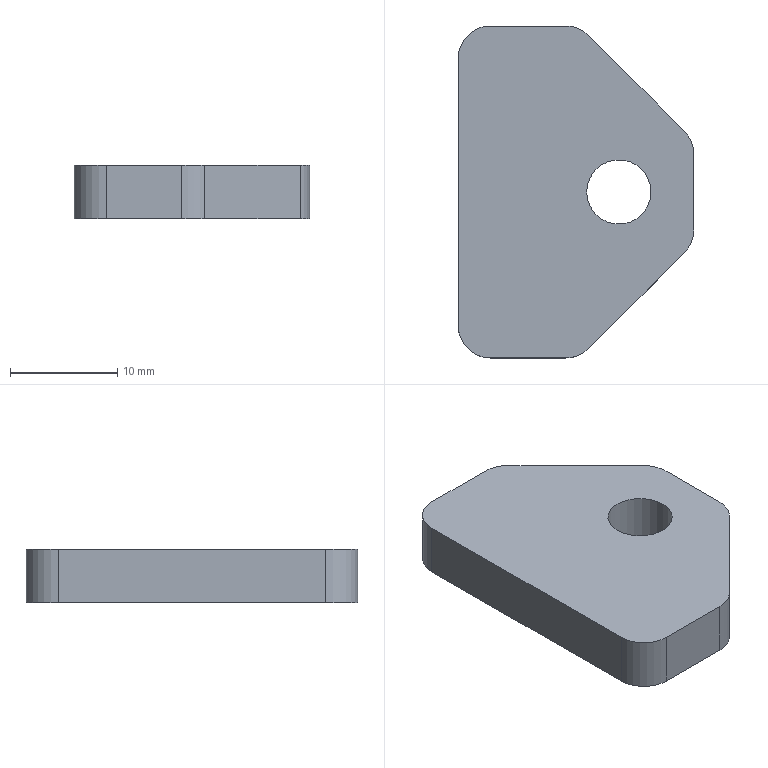Part | NX | features DIE-23 2 | 1 solid | 15 faces | box 22 x 31 x 5 mm | volume 2672 mm3 | plane 8 | cylinder 7 | commonest cylinder face diameters 6 x6 6.007 x1
STEP:
#1=CARTESIAN_POINT('',(2452.36,-823.273,843.716));
#2=VERTEX_POINT('',#1);
#3=CARTESIAN_POINT('',(2445.31,-823.273,843.716));
#4=VERTEX_POINT('',#3);
#5=CARTESIAN_POINT('',(2447.81,-823.273,843.716));
#6=DIRECTION('',(-1.,0.,0.));
#7=VECTOR('',#6,1000.);
#8=LINE('',#5,#7);
#9=EDGE_CURVE('',#2,#4,#8,.T.);
#10=ORIENTED_EDGE('',*,*,#9,.F.);
#11=CARTESIAN_POINT('',(2452.36,-823.273,838.716));
#12=VERTEX_POINT('',#11);
#13=CARTESIAN_POINT('',(2452.36,-823.273,838.716));
#14=DIRECTION('',(0.,0.,1.));
#15=VECTOR('',#14,1000.);
#16=LINE('',#13,#15);
#17=EDGE_CURVE('',#12,#2,#16,.T.);
#18=ORIENTED_EDGE('',*,*,#17,.F.);
#19=CARTESIAN_POINT('',(2445.31,-823.273,838.716));
#20=VERTEX_POINT('',#19);
#21=CARTESIAN_POINT('',(2447.81,-823.273,838.716));
#22=DIRECTION('',(-1.,0.,0.));
#23=VECTOR('',#22,1000.);
#24=LINE('',#21,#23);
#25=EDGE_CURVE('',#12,#20,#24,.T.);
#26=ORIENTED_EDGE('',*,*,#25,.T.);
#27=CARTESIAN_POINT('',(2445.31,-823.273,838.716));
#28=DIRECTION('',(0.,0.,1.));
#29=VECTOR('',#28,1000.);
#30=LINE('',#27,#29);
#31=EDGE_CURVE('',#20,#4,#30,.T.);
#32=ORIENTED_EDGE('',*,*,#31,.T.);
#33=EDGE_LOOP('',(#10,#18,#26,#32));
#34=FACE_BOUND('',#33,.T.);
#35=CARTESIAN_POINT('',(2447.81,-823.273,838.716));
#36=DIRECTION('',(0.,1.,0.));
#37=DIRECTION('',(0.,0.,1.));
#38=AXIS2_PLACEMENT_3D('',#35,#36,#37);
#39=PLANE('',#38);
#40=ADVANCED_FACE('',(#34),#39,.T.);
#41=CARTESIAN_POINT('',(2454.481,-824.152,843.716));
#42=VERTEX_POINT('',#41);
#43=CARTESIAN_POINT('',(2452.36,-826.273,843.716));
#44=DIRECTION('',(0.,0.,-1.));
#45=DIRECTION('',(-1.,0.,0.));
#46=AXIS2_PLACEMENT_3D('',#43,#44,#45);
#47=CIRCLE('',#46,3.);
#48=EDGE_CURVE('',#2,#42,#47,.T.);
#49=ORIENTED_EDGE('',*,*,#48,.T.);
#50=CARTESIAN_POINT('',(2454.481,-824.152,838.716));
#51=VERTEX_POINT('',#50);
#52=CARTESIAN_POINT('',(2454.481,-824.152,838.716));
#53=DIRECTION('',(0.,0.,1.));
#54=VECTOR('',#53,1000.);
#55=LINE('',#52,#54);
#56=EDGE_CURVE('',#51,#42,#55,.T.);
#57=ORIENTED_EDGE('',*,*,#56,.F.);
#58=CARTESIAN_POINT('',(2452.36,-826.273,838.716));
#59=DIRECTION('',(0.,0.,-1.));
#60=DIRECTION('',(-1.,0.,0.));
#61=AXIS2_PLACEMENT_3D('',#58,#59,#60);
#62=CIRCLE('',#61,3.);
#63=EDGE_CURVE('',#12,#51,#62,.T.);
#64=ORIENTED_EDGE('',*,*,#63,.F.);
#65=ORIENTED_EDGE('',*,*,#17,.T.);
#66=EDGE_LOOP('',(#49,#57,#64,#65));
#67=FACE_BOUND('',#66,.T.);
#68=CARTESIAN_POINT('',(2452.36,-826.273,838.716));
#69=DIRECTION('',(0.,0.,1.));
#70=DIRECTION('',(1.,0.,0.));
#71=AXIS2_PLACEMENT_3D('',#68,#69,#70);
#72=CYLINDRICAL_SURFACE('',#71,3.);
#73=ADVANCED_FACE('',(#67),#72,.T.);
#74=CARTESIAN_POINT('',(2463.431,-833.102,843.716));
#75=VERTEX_POINT('',#74);
#76=CARTESIAN_POINT('',(2458.456,-828.127,843.716));
#77=DIRECTION('',(0.7071,-0.7071,0.));
#78=VECTOR('',#77,1000.);
#79=LINE('',#76,#78);
#80=EDGE_CURVE('',#42,#75,#79,.T.);
#81=ORIENTED_EDGE('',*,*,#80,.T.);
#82=CARTESIAN_POINT('',(2463.431,-833.102,838.716));
#83=VERTEX_POINT('',#82);
#84=CARTESIAN_POINT('',(2463.431,-833.102,838.716));
#85=DIRECTION('',(0.,0.,1.));
#86=VECTOR('',#85,1000.);
#87=LINE('',#84,#86);
#88=EDGE_CURVE('',#83,#75,#87,.T.);
#89=ORIENTED_EDGE('',*,*,#88,.F.);
#90=CARTESIAN_POINT('',(2458.456,-828.127,838.716));
#91=DIRECTION('',(0.7071,-0.7071,0.));
#92=VECTOR('',#91,1000.);
#93=LINE('',#90,#92);
#94=EDGE_CURVE('',#51,#83,#93,.T.);
#95=ORIENTED_EDGE('',*,*,#94,.F.);
#96=ORIENTED_EDGE('',*,*,#56,.T.);
#97=EDGE_LOOP('',(#81,#89,#95,#96));
#98=FACE_BOUND('',#97,.T.);
#99=CARTESIAN_POINT('',(2458.456,-828.127,838.716));
#100=DIRECTION('',(-0.7071,-0.7071,0.));
#101=DIRECTION('',(0.7071,-0.7071,0.));
#102=AXIS2_PLACEMENT_3D('',#99,#100,#101);
#103=PLANE('',#102);
#104=ADVANCED_FACE('',(#98),#103,.F.);
#105=CARTESIAN_POINT('',(2464.31,-835.223,843.716));
#106=VERTEX_POINT('',#105);
#107=CARTESIAN_POINT('',(2461.31,-835.223,843.716));
#108=DIRECTION('',(0.,0.,-1.));
#109=DIRECTION('',(-1.,0.,0.));
#110=AXIS2_PLACEMENT_3D('',#107,#108,#109);
#111=CIRCLE('',#110,3.);
#112=EDGE_CURVE('',#75,#106,#111,.T.);
#113=ORIENTED_EDGE('',*,*,#112,.T.);
#114=CARTESIAN_POINT('',(2464.31,-835.223,838.716));
#115=VERTEX_POINT('',#114);
#116=CARTESIAN_POINT('',(2464.31,-835.223,838.716));
#117=DIRECTION('',(0.,0.,1.));
#118=VECTOR('',#117,1000.);
#119=LINE('',#116,#118);
#120=EDGE_CURVE('',#115,#106,#119,.T.);
#121=ORIENTED_EDGE('',*,*,#120,.F.);
#122=CARTESIAN_POINT('',(2461.31,-835.223,838.716));
#123=DIRECTION('',(0.,0.,-1.));
#124=DIRECTION('',(-1.,0.,0.));
#125=AXIS2_PLACEMENT_3D('',#122,#123,#124);
#126=CIRCLE('',#125,3.);
#127=EDGE_CURVE('',#83,#115,#126,.T.);
#128=ORIENTED_EDGE('',*,*,#127,.F.);
#129=ORIENTED_EDGE('',*,*,#88,.T.);
#130=EDGE_LOOP('',(#113,#121,#128,#129));
#131=FACE_BOUND('',#130,.T.);
#132=CARTESIAN_POINT('',(2461.31,-835.223,838.716));
#133=DIRECTION('',(0.,0.,1.));
#134=DIRECTION('',(1.,0.,0.));
#135=AXIS2_PLACEMENT_3D('',#132,#133,#134);
#136=CYLINDRICAL_SURFACE('',#135,3.);
#137=ADVANCED_FACE('',(#131),#136,.T.);
#138=CARTESIAN_POINT('',(2464.31,-842.324,843.716));
#139=VERTEX_POINT('',#138);
#140=CARTESIAN_POINT('',(2464.31,-838.773,843.716));
#141=DIRECTION('',(0.,1.,0.));
#142=VECTOR('',#141,1000.);
#143=LINE('',#140,#142);
#144=EDGE_CURVE('',#139,#106,#143,.T.);
#145=ORIENTED_EDGE('',*,*,#144,.F.);
#146=CARTESIAN_POINT('',(2464.31,-842.324,838.716));
#147=VERTEX_POINT('',#146);
#148=CARTESIAN_POINT('',(2464.31,-842.324,838.716));
#149=DIRECTION('',(0.,0.,1.));
#150=VECTOR('',#149,1000.);
#151=LINE('',#148,#150);
#152=EDGE_CURVE('',#147,#139,#151,.T.);
#153=ORIENTED_EDGE('',*,*,#152,.F.);
#154=CARTESIAN_POINT('',(2464.31,-838.773,838.716));
#155=DIRECTION('',(0.,1.,0.));
#156=VECTOR('',#155,1000.);
#157=LINE('',#154,#156);
#158=EDGE_CURVE('',#147,#115,#157,.T.);
#159=ORIENTED_EDGE('',*,*,#158,.T.);
#160=ORIENTED_EDGE('',*,*,#120,.T.);
#161=EDGE_LOOP('',(#145,#153,#159,#160));
#162=FACE_BOUND('',#161,.T.);
#163=CARTESIAN_POINT('',(2464.31,-838.773,838.716));
#164=DIRECTION('',(1.,0.,0.));
#165=DIRECTION('',(0.,0.,-1.));
#166=AXIS2_PLACEMENT_3D('',#163,#164,#165);
#167=PLANE('',#166);
#168=ADVANCED_FACE('',(#162),#167,.T.);
#169=CARTESIAN_POINT('',(2463.431,-844.445,843.716));
#170=VERTEX_POINT('',#169);
#171=CARTESIAN_POINT('',(2461.31,-842.324,843.716));
#172=DIRECTION('',(0.,0.,-1.));
#173=DIRECTION('',(-1.,0.,0.));
#174=AXIS2_PLACEMENT_3D('',#171,#172,#173);
#175=CIRCLE('',#174,3.);
#176=EDGE_CURVE('',#139,#170,#175,.T.);
#177=ORIENTED_EDGE('',*,*,#176,.T.);
#178=CARTESIAN_POINT('',(2463.431,-844.445,838.716));
#179=VERTEX_POINT('',#178);
#180=CARTESIAN_POINT('',(2463.431,-844.445,838.716));
#181=DIRECTION('',(0.,0.,1.));
#182=VECTOR('',#181,1000.);
#183=LINE('',#180,#182);
#184=EDGE_CURVE('',#179,#170,#183,.T.);
#185=ORIENTED_EDGE('',*,*,#184,.F.);
#186=CARTESIAN_POINT('',(2461.31,-842.324,838.716));
#187=DIRECTION('',(0.,0.,-1.));
#188=DIRECTION('',(-1.,0.,0.));
#189=AXIS2_PLACEMENT_3D('',#186,#187,#188);
#190=CIRCLE('',#189,3.);
#191=EDGE_CURVE('',#147,#179,#190,.T.);
#192=ORIENTED_EDGE('',*,*,#191,.F.);
#193=ORIENTED_EDGE('',*,*,#152,.T.);
#194=EDGE_LOOP('',(#177,#185,#192,#193));
#195=FACE_BOUND('',#194,.T.);
#196=CARTESIAN_POINT('',(2461.31,-842.324,838.716));
#197=DIRECTION('',(0.,0.,1.));
#198=DIRECTION('',(1.,0.,0.));
#199=AXIS2_PLACEMENT_3D('',#196,#197,#198);
#200=CYLINDRICAL_SURFACE('',#199,3.);
#201=ADVANCED_FACE('',(#195),#200,.T.);
#202=CARTESIAN_POINT('',(2454.481,-853.395,843.716));
#203=VERTEX_POINT('',#202);
#204=CARTESIAN_POINT('',(2458.456,-849.42,843.716));
#205=DIRECTION('',(-0.7071,-0.7071,0.));
#206=VECTOR('',#205,1000.);
#207=LINE('',#204,#206);
#208=EDGE_CURVE('',#170,#203,#207,.T.);
#209=ORIENTED_EDGE('',*,*,#208,.T.);
#210=CARTESIAN_POINT('',(2454.481,-853.395,838.716));
#211=VERTEX_POINT('',#210);
#212=CARTESIAN_POINT('',(2454.481,-853.395,838.716));
#213=DIRECTION('',(0.,0.,1.));
#214=VECTOR('',#213,1000.);
#215=LINE('',#212,#214);
#216=EDGE_CURVE('',#211,#203,#215,.T.);
#217=ORIENTED_EDGE('',*,*,#216,.F.);
#218=CARTESIAN_POINT('',(2458.456,-849.42,838.716));
#219=DIRECTION('',(-0.7071,-0.7071,0.));
#220=VECTOR('',#219,1000.);
#221=LINE('',#218,#220);
#222=EDGE_CURVE('',#179,#211,#221,.T.);
#223=ORIENTED_EDGE('',*,*,#222,.F.);
#224=ORIENTED_EDGE('',*,*,#184,.T.);
#225=EDGE_LOOP('',(#209,#217,#223,#224));
#226=FACE_BOUND('',#225,.T.);
#227=CARTESIAN_POINT('',(2458.456,-849.42,838.716));
#228=DIRECTION('',(-0.7071,0.7071,0.));
#229=DIRECTION('',(-0.7071,-0.7071,0.));
#230=AXIS2_PLACEMENT_3D('',#227,#228,#229);
#231=PLANE('',#230);
#232=ADVANCED_FACE('',(#226),#231,.F.);
#233=CARTESIAN_POINT('',(2452.36,-854.273,843.716));
#234=VERTEX_POINT('',#233);
#235=CARTESIAN_POINT('',(2452.36,-851.273,843.716));
#236=DIRECTION('',(0.,0.,-1.));
#237=DIRECTION('',(-1.,0.,0.));
#238=AXIS2_PLACEMENT_3D('',#235,#236,#237);
#239=CIRCLE('',#238,3.);
#240=EDGE_CURVE('',#203,#234,#239,.T.);
#241=ORIENTED_EDGE('',*,*,#240,.T.);
#242=CARTESIAN_POINT('',(2452.36,-854.273,838.716));
#243=VERTEX_POINT('',#242);
#244=CARTESIAN_POINT('',(2452.36,-854.273,838.716));
#245=DIRECTION('',(0.,0.,1.));
#246=VECTOR('',#245,1000.);
#247=LINE('',#244,#246);
#248=EDGE_CURVE('',#243,#234,#247,.T.);
#249=ORIENTED_EDGE('',*,*,#248,.F.);
#250=CARTESIAN_POINT('',(2452.36,-851.273,838.716));
#251=DIRECTION('',(0.,0.,-1.));
#252=DIRECTION('',(-1.,0.,0.));
#253=AXIS2_PLACEMENT_3D('',#250,#251,#252);
#254=CIRCLE('',#253,3.);
#255=EDGE_CURVE('',#211,#243,#254,.T.);
#256=ORIENTED_EDGE('',*,*,#255,.F.);
#257=ORIENTED_EDGE('',*,*,#216,.T.);
#258=EDGE_LOOP('',(#241,#249,#256,#257));
#259=FACE_BOUND('',#258,.T.);
#260=CARTESIAN_POINT('',(2452.36,-851.273,838.716));
#261=DIRECTION('',(0.,0.,1.));
#262=DIRECTION('',(1.,0.,0.));
#263=AXIS2_PLACEMENT_3D('',#260,#261,#262);
#264=CYLINDRICAL_SURFACE('',#263,3.);
#265=ADVANCED_FACE('',(#259),#264,.T.);
#266=CARTESIAN_POINT('',(2445.31,-854.273,843.716));
#267=VERTEX_POINT('',#266);
#268=CARTESIAN_POINT('',(2447.81,-854.273,843.716));
#269=DIRECTION('',(1.,0.,0.));
#270=VECTOR('',#269,1000.);
#271=LINE('',#268,#270);
#272=EDGE_CURVE('',#267,#234,#271,.T.);
#273=ORIENTED_EDGE('',*,*,#272,.F.);
#274=CARTESIAN_POINT('',(2445.31,-854.273,838.716));
#275=VERTEX_POINT('',#274);
#276=CARTESIAN_POINT('',(2445.31,-854.273,838.716));
#277=DIRECTION('',(0.,0.,1.));
#278=VECTOR('',#277,1000.);
#279=LINE('',#276,#278);
#280=EDGE_CURVE('',#275,#267,#279,.T.);
#281=ORIENTED_EDGE('',*,*,#280,.F.);
#282=CARTESIAN_POINT('',(2447.81,-854.273,838.716));
#283=DIRECTION('',(1.,0.,0.));
#284=VECTOR('',#283,1000.);
#285=LINE('',#282,#284);
#286=EDGE_CURVE('',#275,#243,#285,.T.);
#287=ORIENTED_EDGE('',*,*,#286,.T.);
#288=ORIENTED_EDGE('',*,*,#248,.T.);
#289=EDGE_LOOP('',(#273,#281,#287,#288));
#290=FACE_BOUND('',#289,.T.);
#291=CARTESIAN_POINT('',(2447.81,-854.273,838.716));
#292=DIRECTION('',(0.,-1.,0.));
#293=DIRECTION('',(0.,0.,-1.));
#294=AXIS2_PLACEMENT_3D('',#291,#292,#293);
#295=PLANE('',#294);
#296=ADVANCED_FACE('',(#290),#295,.T.);
#297=CARTESIAN_POINT('',(2442.31,-851.273,843.716));
#298=VERTEX_POINT('',#297);
#299=CARTESIAN_POINT('',(2445.31,-851.273,843.716));
#300=DIRECTION('',(0.,0.,-1.));
#301=DIRECTION('',(-1.,0.,0.));
#302=AXIS2_PLACEMENT_3D('',#299,#300,#301);
#303=CIRCLE('',#302,3.);
#304=EDGE_CURVE('',#267,#298,#303,.T.);
#305=ORIENTED_EDGE('',*,*,#304,.T.);
#306=CARTESIAN_POINT('',(2442.31,-851.273,838.716));
#307=VERTEX_POINT('',#306);
#308=CARTESIAN_POINT('',(2442.31,-851.273,838.716));
#309=DIRECTION('',(0.,0.,1.));
#310=VECTOR('',#309,1000.);
#311=LINE('',#308,#310);
#312=EDGE_CURVE('',#307,#298,#311,.T.);
#313=ORIENTED_EDGE('',*,*,#312,.F.);
#314=CARTESIAN_POINT('',(2445.31,-851.273,838.716));
#315=DIRECTION('',(0.,0.,-1.));
#316=DIRECTION('',(-1.,0.,0.));
#317=AXIS2_PLACEMENT_3D('',#314,#315,#316);
#318=CIRCLE('',#317,3.);
#319=EDGE_CURVE('',#275,#307,#318,.T.);
#320=ORIENTED_EDGE('',*,*,#319,.F.);
#321=ORIENTED_EDGE('',*,*,#280,.T.);
#322=EDGE_LOOP('',(#305,#313,#320,#321));
#323=FACE_BOUND('',#322,.T.);
#324=CARTESIAN_POINT('',(2445.31,-851.273,838.716));
#325=DIRECTION('',(0.,0.,1.));
#326=DIRECTION('',(1.,0.,0.));
#327=AXIS2_PLACEMENT_3D('',#324,#325,#326);
#328=CYLINDRICAL_SURFACE('',#327,3.);
#329=ADVANCED_FACE('',(#323),#328,.T.);
#330=CARTESIAN_POINT('',(2442.31,-826.273,843.716));
#331=VERTEX_POINT('',#330);
#332=CARTESIAN_POINT('',(2442.31,-838.773,843.716));
#333=DIRECTION('',(0.,-1.,0.));
#334=VECTOR('',#333,1000.);
#335=LINE('',#332,#334);
#336=EDGE_CURVE('',#331,#298,#335,.T.);
#337=ORIENTED_EDGE('',*,*,#336,.F.);
#338=CARTESIAN_POINT('',(2442.31,-826.273,838.716));
#339=VERTEX_POINT('',#338);
#340=CARTESIAN_POINT('',(2442.31,-826.273,838.716));
#341=DIRECTION('',(0.,0.,1.));
#342=VECTOR('',#341,1000.);
#343=LINE('',#340,#342);
#344=EDGE_CURVE('',#339,#331,#343,.T.);
#345=ORIENTED_EDGE('',*,*,#344,.F.);
#346=CARTESIAN_POINT('',(2442.31,-838.773,838.716));
#347=DIRECTION('',(0.,-1.,0.));
#348=VECTOR('',#347,1000.);
#349=LINE('',#346,#348);
#350=EDGE_CURVE('',#339,#307,#349,.T.);
#351=ORIENTED_EDGE('',*,*,#350,.T.);
#352=ORIENTED_EDGE('',*,*,#312,.T.);
#353=EDGE_LOOP('',(#337,#345,#351,#352));
#354=FACE_BOUND('',#353,.T.);
#355=CARTESIAN_POINT('',(2442.31,-838.773,838.716));
#356=DIRECTION('',(-1.,0.,0.));
#357=DIRECTION('',(0.,0.,1.));
#358=AXIS2_PLACEMENT_3D('',#355,#356,#357);
#359=PLANE('',#358);
#360=ADVANCED_FACE('',(#354),#359,.T.);
#361=CARTESIAN_POINT('',(2454.306,-838.773,838.716));
#362=VERTEX_POINT('',#361);
#363=CARTESIAN_POINT('',(2457.31,-838.773,838.716));
#364=DIRECTION('',(0.,0.,-1.));
#365=DIRECTION('',(-1.,0.,0.));
#366=AXIS2_PLACEMENT_3D('',#363,#364,#365);
#367=CIRCLE('',#366,3.003);
#368=EDGE_CURVE('',#362,#362,#367,.T.);
#369=ORIENTED_EDGE('',*,*,#368,.T.);
#370=EDGE_LOOP('',(#369));
#371=FACE_BOUND('',#370,.T.);
#372=CARTESIAN_POINT('',(2454.306,-838.773,843.716));
#373=VERTEX_POINT('',#372);
#374=CARTESIAN_POINT('',(2457.31,-838.773,843.716));
#375=DIRECTION('',(0.,0.,-1.));
#376=DIRECTION('',(-1.,0.,0.));
#377=AXIS2_PLACEMENT_3D('',#374,#375,#376);
#378=CIRCLE('',#377,3.003);
#379=EDGE_CURVE('',#373,#373,#378,.T.);
#380=ORIENTED_EDGE('',*,*,#379,.F.);
#381=EDGE_LOOP('',(#380));
#382=FACE_BOUND('',#381,.T.);
#383=CARTESIAN_POINT('',(2457.31,-838.773,838.716));
#384=DIRECTION('',(0.,0.,1.));
#385=DIRECTION('',(1.,0.,0.));
#386=AXIS2_PLACEMENT_3D('',#383,#384,#385);
#387=CYLINDRICAL_SURFACE('',#386,3.003);
#388=ADVANCED_FACE('',(#371,#382),#387,.F.);
#389=CARTESIAN_POINT('',(2445.31,-826.273,843.716));
#390=DIRECTION('',(0.,0.,-1.));
#391=DIRECTION('',(-1.,0.,0.));
#392=AXIS2_PLACEMENT_3D('',#389,#390,#391);
#393=CIRCLE('',#392,3.);
#394=EDGE_CURVE('',#331,#4,#393,.T.);
#395=ORIENTED_EDGE('',*,*,#394,.T.);
#396=ORIENTED_EDGE('',*,*,#31,.F.);
#397=CARTESIAN_POINT('',(2445.31,-826.273,838.716));
#398=DIRECTION('',(0.,0.,-1.));
#399=DIRECTION('',(-1.,0.,0.));
#400=AXIS2_PLACEMENT_3D('',#397,#398,#399);
#401=CIRCLE('',#400,3.);
#402=EDGE_CURVE('',#339,#20,#401,.T.);
#403=ORIENTED_EDGE('',*,*,#402,.F.);
#404=ORIENTED_EDGE('',*,*,#344,.T.);
#405=EDGE_LOOP('',(#395,#396,#403,#404));
#406=FACE_BOUND('',#405,.T.);
#407=CARTESIAN_POINT('',(2445.31,-826.273,838.716));
#408=DIRECTION('',(0.,0.,1.));
#409=DIRECTION('',(1.,0.,0.));
#410=AXIS2_PLACEMENT_3D('',#407,#408,#409);
#411=CYLINDRICAL_SURFACE('',#410,3.);
#412=ADVANCED_FACE('',(#406),#411,.T.);
#413=ORIENTED_EDGE('',*,*,#368,.F.);
#414=EDGE_LOOP('',(#413));
#415=FACE_BOUND('',#414,.T.);
#416=ORIENTED_EDGE('',*,*,#25,.F.);
#417=ORIENTED_EDGE('',*,*,#63,.T.);
#418=ORIENTED_EDGE('',*,*,#94,.T.);
#419=ORIENTED_EDGE('',*,*,#127,.T.);
#420=ORIENTED_EDGE('',*,*,#158,.F.);
#421=ORIENTED_EDGE('',*,*,#191,.T.);
#422=ORIENTED_EDGE('',*,*,#222,.T.);
#423=ORIENTED_EDGE('',*,*,#255,.T.);
#424=ORIENTED_EDGE('',*,*,#286,.F.);
#425=ORIENTED_EDGE('',*,*,#319,.T.);
#426=ORIENTED_EDGE('',*,*,#350,.F.);
#427=ORIENTED_EDGE('',*,*,#402,.T.);
#428=EDGE_LOOP('',(#416,#417,#418,#419,#420,#421,#422,#423,#424,#425,#426,#427));
#429=FACE_BOUND('',#428,.T.);
#430=CARTESIAN_POINT('',(2447.81,-838.773,838.716));
#431=DIRECTION('',(0.,0.,-1.));
#432=DIRECTION('',(-1.,0.,0.));
#433=AXIS2_PLACEMENT_3D('',#430,#431,#432);
#434=PLANE('',#433);
#435=ADVANCED_FACE('',(#415,#429),#434,.T.);
#436=ORIENTED_EDGE('',*,*,#379,.T.);
#437=EDGE_LOOP('',(#436));
#438=FACE_BOUND('',#437,.T.);
#439=ORIENTED_EDGE('',*,*,#9,.T.);
#440=ORIENTED_EDGE('',*,*,#394,.F.);
#441=ORIENTED_EDGE('',*,*,#336,.T.);
#442=ORIENTED_EDGE('',*,*,#304,.F.);
#443=ORIENTED_EDGE('',*,*,#272,.T.);
#444=ORIENTED_EDGE('',*,*,#240,.F.);
#445=ORIENTED_EDGE('',*,*,#208,.F.);
#446=ORIENTED_EDGE('',*,*,#176,.F.);
#447=ORIENTED_EDGE('',*,*,#144,.T.);
#448=ORIENTED_EDGE('',*,*,#112,.F.);
#449=ORIENTED_EDGE('',*,*,#80,.F.);
#450=ORIENTED_EDGE('',*,*,#48,.F.);
#451=EDGE_LOOP('',(#439,#440,#441,#442,#443,#444,#445,#446,#447,#448,#449,#450));
#452=FACE_BOUND('',#451,.T.);
#453=CARTESIAN_POINT('',(2447.81,-838.773,843.716));
#454=DIRECTION('',(0.,0.,-1.));
#455=DIRECTION('',(-1.,0.,0.));
#456=AXIS2_PLACEMENT_3D('',#453,#454,#455);
#457=PLANE('',#456);
#458=ADVANCED_FACE('',(#438,#452),#457,.F.);
#459=CLOSED_SHELL('',(#40,#73,#104,#137,#168,#201,#232,#265,#296,#329,#360,#388,#412,#435,#458));
#460=MANIFOLD_SOLID_BREP('',#459);
#461=(LENGTH_UNIT()NAMED_UNIT(*)SI_UNIT(.MILLI.,.METRE.));
#462=UNCERTAINTY_MEASURE_WITH_UNIT(LENGTH_MEASURE(0.00001),#461,'','');
#463=(NAMED_UNIT(*)PLANE_ANGLE_UNIT()SI_UNIT($,.RADIAN.));
#464=(NAMED_UNIT(*)SI_UNIT($,.STERADIAN.)SOLID_ANGLE_UNIT());
#465=(GEOMETRIC_REPRESENTATION_CONTEXT(3)GLOBAL_UNCERTAINTY_ASSIGNED_CONTEXT((#462))GLOBAL_UNIT_ASSIGNED_CONTEXT((#461,#463,#464))REPRESENTATION_CONTEXT('',''));
#466=ADVANCED_BREP_SHAPE_REPRESENTATION('',(#460),#465);